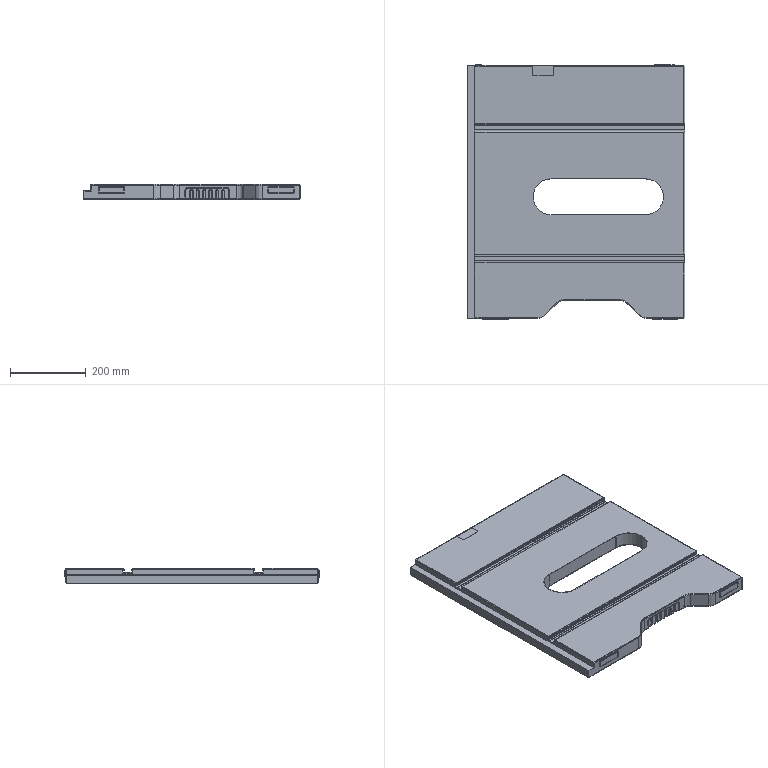Part | STEP file | DEWALT-DWE7492-B22 | 1 solid | 841 faces | box 575 x 674 x 40 mm | volume 781734 mm3 | cylinder 288 | plane 285 | torus 152 | spline 60 | other 36 | cone 20 | commonest cylinder face diameters 1 x80 2 x68 4 x56 5 x34 3 x18 6 x8